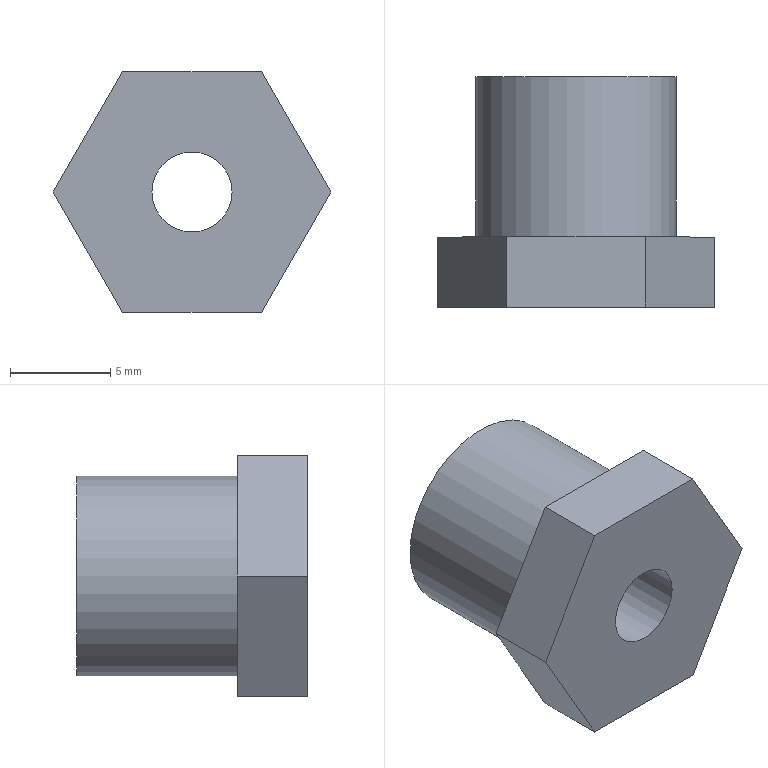Part | STEP file | 1-06.4 | 1 solid | 11 faces | box 13.856 x 11.5 x 12 mm | volume 920.282 mm3 | plane 9 | cylinder 2 | commonest cylinder face diameters 4 x1 10 x1
STEP:
#1=CARTESIAN_POINT('',(0.,0.,0.));
#2=DIRECTION('',(0.,0.,1.));
#3=DIRECTION('',(1.,0.,0.));
#4=AXIS2_PLACEMENT_3D('',#1,#2,#3);
#5=CARTESIAN_POINT('',(-3.464,0.,6.));
#6=VERTEX_POINT('',#5);
#7=CARTESIAN_POINT('',(3.464,0.,6.));
#8=VERTEX_POINT('',#7);
#9=CARTESIAN_POINT('',(-3.464,0.,6.));
#10=DIRECTION('',(1.,0.,0.));
#11=VECTOR('',#10,1.);
#12=LINE('',#9,#11);
#13=CARTESIAN_POINT('',(0.,-1.75,6.));
#14=DIRECTION('',(0.,0.,-1.));
#15=DIRECTION('',(1.,0.,0.));
#16=AXIS2_PLACEMENT_3D('',#13,#14,#15);
#17=PLANE('',#16);
#18=CARTESIAN_POINT('',(-3.464,-1.75));
#19=DIRECTION('',(1.,0.));
#20=VECTOR('',#19,1.);
#21=LINE('',#18,#20);
#22=(GEOMETRIC_REPRESENTATION_CONTEXT(2)PARAMETRIC_REPRESENTATION_CONTEXT()REPRESENTATION_CONTEXT('',''));
#23=DEFINITIONAL_REPRESENTATION('',(#21),#22);
#24=PCURVE('',#17,#23);
#25=CARTESIAN_POINT('',(0.,0.,-0.9282));
#26=DIRECTION('',(0.,1.,0.));
#27=DIRECTION('',(1.,0.,0.));
#28=AXIS2_PLACEMENT_3D('',#25,#26,#27);
#29=PLANE('',#28);
#30=CARTESIAN_POINT('',(-3.464,-6.928));
#31=DIRECTION('',(1.,0.));
#32=VECTOR('',#31,1.);
#33=LINE('',#30,#32);
#34=(GEOMETRIC_REPRESENTATION_CONTEXT(2)PARAMETRIC_REPRESENTATION_CONTEXT()REPRESENTATION_CONTEXT('',''));
#35=DEFINITIONAL_REPRESENTATION('',(#33),#34);
#36=PCURVE('',#29,#35);
#37=SURFACE_CURVE('',#12,(#24,#36),.PCURVE_S1.);
#38=EDGE_CURVE('',#6,#8,#37,.T.);
#39=ORIENTED_EDGE('',*,*,#38,.T.);
#40=CARTESIAN_POINT('',(3.464,-3.5,6.));
#41=VERTEX_POINT('',#40);
#42=CARTESIAN_POINT('',(3.464,0.,6.));
#43=DIRECTION('',(0.,-1.,0.));
#44=VECTOR('',#43,1.);
#45=LINE('',#42,#44);
#46=CARTESIAN_POINT('',(3.464,-1.75));
#47=DIRECTION('',(0.,1.));
#48=VECTOR('',#47,1.);
#49=LINE('',#46,#48);
#50=(GEOMETRIC_REPRESENTATION_CONTEXT(2)PARAMETRIC_REPRESENTATION_CONTEXT()REPRESENTATION_CONTEXT('',''));
#51=DEFINITIONAL_REPRESENTATION('',(#49),#50);
#52=PCURVE('',#17,#51);
#53=CARTESIAN_POINT('',(5.196,-1.75,3.));
#54=DIRECTION('',(-0.866,0.,-0.5));
#55=DIRECTION('',(0.5,0.,-0.866));
#56=AXIS2_PLACEMENT_3D('',#53,#54,#55);
#57=PLANE('',#56);
#58=CARTESIAN_POINT('',(-3.464,-1.75));
#59=DIRECTION('',(0.,1.));
#60=VECTOR('',#59,1.);
#61=LINE('',#58,#60);
#62=(GEOMETRIC_REPRESENTATION_CONTEXT(2)PARAMETRIC_REPRESENTATION_CONTEXT()REPRESENTATION_CONTEXT('',''));
#63=DEFINITIONAL_REPRESENTATION('',(#61),#62);
#64=PCURVE('',#57,#63);
#65=SURFACE_CURVE('',#45,(#52,#64),.PCURVE_S1.);
#66=EDGE_CURVE('',#8,#41,#65,.T.);
#67=ORIENTED_EDGE('',*,*,#66,.T.);
#68=CARTESIAN_POINT('',(-3.464,-3.5,6.));
#69=VERTEX_POINT('',#68);
#70=CARTESIAN_POINT('',(-3.464,-3.5,6.));
#71=DIRECTION('',(1.,0.,0.));
#72=VECTOR('',#71,1.);
#73=LINE('',#70,#72);
#74=CARTESIAN_POINT('',(-3.464,1.75));
#75=DIRECTION('',(1.,0.));
#76=VECTOR('',#75,1.);
#77=LINE('',#74,#76);
#78=(GEOMETRIC_REPRESENTATION_CONTEXT(2)PARAMETRIC_REPRESENTATION_CONTEXT()REPRESENTATION_CONTEXT('',''));
#79=DEFINITIONAL_REPRESENTATION('',(#77),#78);
#80=PCURVE('',#17,#79);
#81=CARTESIAN_POINT('',(0.,-3.5,-0.9282));
#82=DIRECTION('',(0.,1.,0.));
#83=DIRECTION('',(1.,0.,0.));
#84=AXIS2_PLACEMENT_3D('',#81,#82,#83);
#85=PLANE('',#84);
#86=CARTESIAN_POINT('',(-3.464,-6.928));
#87=DIRECTION('',(1.,0.));
#88=VECTOR('',#87,1.);
#89=LINE('',#86,#88);
#90=(GEOMETRIC_REPRESENTATION_CONTEXT(2)PARAMETRIC_REPRESENTATION_CONTEXT()REPRESENTATION_CONTEXT('',''));
#91=DEFINITIONAL_REPRESENTATION('',(#89),#90);
#92=PCURVE('',#85,#91);
#93=SURFACE_CURVE('',#73,(#80,#92),.PCURVE_S1.);
#94=EDGE_CURVE('',#69,#41,#93,.T.);
#95=ORIENTED_EDGE('',*,*,#94,.F.);
#96=CARTESIAN_POINT('',(-3.464,0.,6.));
#97=DIRECTION('',(0.,-1.,0.));
#98=VECTOR('',#97,1.);
#99=LINE('',#96,#98);
#100=CARTESIAN_POINT('',(-3.464,-1.75));
#101=DIRECTION('',(0.,1.));
#102=VECTOR('',#101,1.);
#103=LINE('',#100,#102);
#104=(GEOMETRIC_REPRESENTATION_CONTEXT(2)PARAMETRIC_REPRESENTATION_CONTEXT()REPRESENTATION_CONTEXT('',''));
#105=DEFINITIONAL_REPRESENTATION('',(#103),#104);
#106=PCURVE('',#17,#105);
#107=CARTESIAN_POINT('',(-5.196,-1.75,3.));
#108=DIRECTION('',(0.866,0.,-0.5));
#109=DIRECTION('',(0.5,0.,0.866));
#110=AXIS2_PLACEMENT_3D('',#107,#108,#109);
#111=PLANE('',#110);
#112=CARTESIAN_POINT('',(3.464,-1.75));
#113=DIRECTION('',(0.,1.));
#114=VECTOR('',#113,1.);
#115=LINE('',#112,#114);
#116=(GEOMETRIC_REPRESENTATION_CONTEXT(2)PARAMETRIC_REPRESENTATION_CONTEXT()REPRESENTATION_CONTEXT('',''));
#117=DEFINITIONAL_REPRESENTATION('',(#115),#116);
#118=PCURVE('',#111,#117);
#119=SURFACE_CURVE('',#99,(#106,#118),.PCURVE_S1.);
#120=EDGE_CURVE('',#6,#69,#119,.T.);
#121=ORIENTED_EDGE('',*,*,#120,.F.);
#122=EDGE_LOOP('',(#39,#67,#95,#121));
#123=FACE_BOUND('',#122,.F.);
#124=ADVANCED_FACE('',(#123),#17,.F.);
#125=CARTESIAN_POINT('',(6.928,0.,0.));
#126=VERTEX_POINT('',#125);
#127=CARTESIAN_POINT('',(3.464,0.,6.));
#128=DIRECTION('',(0.5,0.,-0.866));
#129=VECTOR('',#128,1.);
#130=LINE('',#127,#129);
#131=CARTESIAN_POINT('',(-3.464,-1.75));
#132=DIRECTION('',(1.,0.));
#133=VECTOR('',#132,1.);
#134=LINE('',#131,#133);
#135=(GEOMETRIC_REPRESENTATION_CONTEXT(2)PARAMETRIC_REPRESENTATION_CONTEXT()REPRESENTATION_CONTEXT('',''));
#136=DEFINITIONAL_REPRESENTATION('',(#134),#135);
#137=PCURVE('',#57,#136);
#138=CARTESIAN_POINT('',(3.464,-6.928));
#139=DIRECTION('',(0.5,0.866));
#140=VECTOR('',#139,1.);
#141=LINE('',#138,#140);
#142=(GEOMETRIC_REPRESENTATION_CONTEXT(2)PARAMETRIC_REPRESENTATION_CONTEXT()REPRESENTATION_CONTEXT('',''));
#143=DEFINITIONAL_REPRESENTATION('',(#141),#142);
#144=PCURVE('',#29,#143);
#145=SURFACE_CURVE('',#130,(#137,#144),.PCURVE_S1.);
#146=EDGE_CURVE('',#8,#126,#145,.T.);
#147=ORIENTED_EDGE('',*,*,#146,.T.);
#148=CARTESIAN_POINT('',(6.928,-3.5,0.));
#149=VERTEX_POINT('',#148);
#150=CARTESIAN_POINT('',(6.928,0.,0.));
#151=DIRECTION('',(0.,-1.,0.));
#152=VECTOR('',#151,1.);
#153=LINE('',#150,#152);
#154=CARTESIAN_POINT('',(3.464,-1.75));
#155=DIRECTION('',(0.,1.));
#156=VECTOR('',#155,1.);
#157=LINE('',#154,#156);
#158=(GEOMETRIC_REPRESENTATION_CONTEXT(2)PARAMETRIC_REPRESENTATION_CONTEXT()REPRESENTATION_CONTEXT('',''));
#159=DEFINITIONAL_REPRESENTATION('',(#157),#158);
#160=PCURVE('',#57,#159);
#161=CARTESIAN_POINT('',(5.196,-1.75,-3.));
#162=DIRECTION('',(-0.866,0.,0.5));
#163=DIRECTION('',(-0.5,0.,-0.866));
#164=AXIS2_PLACEMENT_3D('',#161,#162,#163);
#165=PLANE('',#164);
#166=CARTESIAN_POINT('',(-3.464,-1.75));
#167=DIRECTION('',(0.,1.));
#168=VECTOR('',#167,1.);
#169=LINE('',#166,#168);
#170=(GEOMETRIC_REPRESENTATION_CONTEXT(2)PARAMETRIC_REPRESENTATION_CONTEXT()REPRESENTATION_CONTEXT('',''));
#171=DEFINITIONAL_REPRESENTATION('',(#169),#170);
#172=PCURVE('',#165,#171);
#173=SURFACE_CURVE('',#153,(#160,#172),.PCURVE_S1.);
#174=EDGE_CURVE('',#126,#149,#173,.T.);
#175=ORIENTED_EDGE('',*,*,#174,.T.);
#176=CARTESIAN_POINT('',(3.464,-3.5,6.));
#177=DIRECTION('',(0.5,0.,-0.866));
#178=VECTOR('',#177,1.);
#179=LINE('',#176,#178);
#180=CARTESIAN_POINT('',(-3.464,1.75));
#181=DIRECTION('',(1.,0.));
#182=VECTOR('',#181,1.);
#183=LINE('',#180,#182);
#184=(GEOMETRIC_REPRESENTATION_CONTEXT(2)PARAMETRIC_REPRESENTATION_CONTEXT()REPRESENTATION_CONTEXT('',''));
#185=DEFINITIONAL_REPRESENTATION('',(#183),#184);
#186=PCURVE('',#57,#185);
#187=CARTESIAN_POINT('',(3.464,-6.928));
#188=DIRECTION('',(0.5,0.866));
#189=VECTOR('',#188,1.);
#190=LINE('',#187,#189);
#191=(GEOMETRIC_REPRESENTATION_CONTEXT(2)PARAMETRIC_REPRESENTATION_CONTEXT()REPRESENTATION_CONTEXT('',''));
#192=DEFINITIONAL_REPRESENTATION('',(#190),#191);
#193=PCURVE('',#85,#192);
#194=SURFACE_CURVE('',#179,(#186,#193),.PCURVE_S1.);
#195=EDGE_CURVE('',#41,#149,#194,.T.);
#196=ORIENTED_EDGE('',*,*,#195,.F.);
#197=ORIENTED_EDGE('',*,*,#66,.F.);
#198=EDGE_LOOP('',(#147,#175,#196,#197));
#199=FACE_BOUND('',#198,.F.);
#200=ADVANCED_FACE('',(#199),#57,.F.);
#201=CARTESIAN_POINT('',(3.464,0.,-6.));
#202=VERTEX_POINT('',#201);
#203=CARTESIAN_POINT('',(6.928,0.,0.));
#204=DIRECTION('',(-0.5,0.,-0.866));
#205=VECTOR('',#204,1.);
#206=LINE('',#203,#205);
#207=CARTESIAN_POINT('',(-3.464,-1.75));
#208=DIRECTION('',(1.,0.));
#209=VECTOR('',#208,1.);
#210=LINE('',#207,#209);
#211=(GEOMETRIC_REPRESENTATION_CONTEXT(2)PARAMETRIC_REPRESENTATION_CONTEXT()REPRESENTATION_CONTEXT('',''));
#212=DEFINITIONAL_REPRESENTATION('',(#210),#211);
#213=PCURVE('',#165,#212);
#214=CARTESIAN_POINT('',(6.928,-0.9282));
#215=DIRECTION('',(-0.5,0.866));
#216=VECTOR('',#215,1.);
#217=LINE('',#214,#216);
#218=(GEOMETRIC_REPRESENTATION_CONTEXT(2)PARAMETRIC_REPRESENTATION_CONTEXT()REPRESENTATION_CONTEXT('',''));
#219=DEFINITIONAL_REPRESENTATION('',(#217),#218);
#220=PCURVE('',#29,#219);
#221=SURFACE_CURVE('',#206,(#213,#220),.PCURVE_S1.);
#222=EDGE_CURVE('',#126,#202,#221,.T.);
#223=ORIENTED_EDGE('',*,*,#222,.T.);
#224=CARTESIAN_POINT('',(3.464,-3.5,-6.));
#225=VERTEX_POINT('',#224);
#226=CARTESIAN_POINT('',(3.464,0.,-6.));
#227=DIRECTION('',(0.,-1.,0.));
#228=VECTOR('',#227,1.);
#229=LINE('',#226,#228);
#230=CARTESIAN_POINT('',(3.464,-1.75));
#231=DIRECTION('',(0.,1.));
#232=VECTOR('',#231,1.);
#233=LINE('',#230,#232);
#234=(GEOMETRIC_REPRESENTATION_CONTEXT(2)PARAMETRIC_REPRESENTATION_CONTEXT()REPRESENTATION_CONTEXT('',''));
#235=DEFINITIONAL_REPRESENTATION('',(#233),#234);
#236=PCURVE('',#165,#235);
#237=CARTESIAN_POINT('',(0.,-1.75,-6.));
#238=DIRECTION('',(0.,0.,1.));
#239=DIRECTION('',(-1.,0.,0.));
#240=AXIS2_PLACEMENT_3D('',#237,#238,#239);
#241=PLANE('',#240);
#242=CARTESIAN_POINT('',(-3.464,-1.75));
#243=DIRECTION('',(0.,1.));
#244=VECTOR('',#243,1.);
#245=LINE('',#242,#244);
#246=(GEOMETRIC_REPRESENTATION_CONTEXT(2)PARAMETRIC_REPRESENTATION_CONTEXT()REPRESENTATION_CONTEXT('',''));
#247=DEFINITIONAL_REPRESENTATION('',(#245),#246);
#248=PCURVE('',#241,#247);
#249=SURFACE_CURVE('',#229,(#236,#248),.PCURVE_S1.);
#250=EDGE_CURVE('',#202,#225,#249,.T.);
#251=ORIENTED_EDGE('',*,*,#250,.T.);
#252=CARTESIAN_POINT('',(6.928,-3.5,0.));
#253=DIRECTION('',(-0.5,0.,-0.866));
#254=VECTOR('',#253,1.);
#255=LINE('',#252,#254);
#256=CARTESIAN_POINT('',(-3.464,1.75));
#257=DIRECTION('',(1.,0.));
#258=VECTOR('',#257,1.);
#259=LINE('',#256,#258);
#260=(GEOMETRIC_REPRESENTATION_CONTEXT(2)PARAMETRIC_REPRESENTATION_CONTEXT()REPRESENTATION_CONTEXT('',''));
#261=DEFINITIONAL_REPRESENTATION('',(#259),#260);
#262=PCURVE('',#165,#261);
#263=CARTESIAN_POINT('',(6.928,-0.9282));
#264=DIRECTION('',(-0.5,0.866));
#265=VECTOR('',#264,1.);
#266=LINE('',#263,#265);
#267=(GEOMETRIC_REPRESENTATION_CONTEXT(2)PARAMETRIC_REPRESENTATION_CONTEXT()REPRESENTATION_CONTEXT('',''));
#268=DEFINITIONAL_REPRESENTATION('',(#266),#267);
#269=PCURVE('',#85,#268);
#270=SURFACE_CURVE('',#255,(#262,#269),.PCURVE_S1.);
#271=EDGE_CURVE('',#149,#225,#270,.T.);
#272=ORIENTED_EDGE('',*,*,#271,.F.);
#273=ORIENTED_EDGE('',*,*,#174,.F.);
#274=EDGE_LOOP('',(#223,#251,#272,#273));
#275=FACE_BOUND('',#274,.F.);
#276=ADVANCED_FACE('',(#275),#165,.F.);
#277=CARTESIAN_POINT('',(-3.464,0.,-6.));
#278=VERTEX_POINT('',#277);
#279=CARTESIAN_POINT('',(3.464,0.,-6.));
#280=DIRECTION('',(-1.,0.,0.));
#281=VECTOR('',#280,1.);
#282=LINE('',#279,#281);
#283=CARTESIAN_POINT('',(-3.464,-1.75));
#284=DIRECTION('',(1.,0.));
#285=VECTOR('',#284,1.);
#286=LINE('',#283,#285);
#287=(GEOMETRIC_REPRESENTATION_CONTEXT(2)PARAMETRIC_REPRESENTATION_CONTEXT()REPRESENTATION_CONTEXT('',''));
#288=DEFINITIONAL_REPRESENTATION('',(#286),#287);
#289=PCURVE('',#241,#288);
#290=CARTESIAN_POINT('',(3.464,5.072));
#291=DIRECTION('',(-1.,0.));
#292=VECTOR('',#291,1.);
#293=LINE('',#290,#292);
#294=(GEOMETRIC_REPRESENTATION_CONTEXT(2)PARAMETRIC_REPRESENTATION_CONTEXT()REPRESENTATION_CONTEXT('',''));
#295=DEFINITIONAL_REPRESENTATION('',(#293),#294);
#296=PCURVE('',#29,#295);
#297=SURFACE_CURVE('',#282,(#289,#296),.PCURVE_S1.);
#298=EDGE_CURVE('',#202,#278,#297,.T.);
#299=ORIENTED_EDGE('',*,*,#298,.T.);
#300=CARTESIAN_POINT('',(-3.464,-3.5,-6.));
#301=VERTEX_POINT('',#300);
#302=CARTESIAN_POINT('',(-3.464,0.,-6.));
#303=DIRECTION('',(0.,-1.,0.));
#304=VECTOR('',#303,1.);
#305=LINE('',#302,#304);
#306=CARTESIAN_POINT('',(3.464,-1.75));
#307=DIRECTION('',(0.,1.));
#308=VECTOR('',#307,1.);
#309=LINE('',#306,#308);
#310=(GEOMETRIC_REPRESENTATION_CONTEXT(2)PARAMETRIC_REPRESENTATION_CONTEXT()REPRESENTATION_CONTEXT('',''));
#311=DEFINITIONAL_REPRESENTATION('',(#309),#310);
#312=PCURVE('',#241,#311);
#313=CARTESIAN_POINT('',(-5.196,-1.75,-3.));
#314=DIRECTION('',(0.866,0.,0.5));
#315=DIRECTION('',(-0.5,0.,0.866));
#316=AXIS2_PLACEMENT_3D('',#313,#314,#315);
#317=PLANE('',#316);
#318=CARTESIAN_POINT('',(-3.464,-1.75));
#319=DIRECTION('',(0.,1.));
#320=VECTOR('',#319,1.);
#321=LINE('',#318,#320);
#322=(GEOMETRIC_REPRESENTATION_CONTEXT(2)PARAMETRIC_REPRESENTATION_CONTEXT()REPRESENTATION_CONTEXT('',''));
#323=DEFINITIONAL_REPRESENTATION('',(#321),#322);
#324=PCURVE('',#317,#323);
#325=SURFACE_CURVE('',#305,(#312,#324),.PCURVE_S1.);
#326=EDGE_CURVE('',#278,#301,#325,.T.);
#327=ORIENTED_EDGE('',*,*,#326,.T.);
#328=CARTESIAN_POINT('',(3.464,-3.5,-6.));
#329=DIRECTION('',(-1.,0.,0.));
#330=VECTOR('',#329,1.);
#331=LINE('',#328,#330);
#332=CARTESIAN_POINT('',(-3.464,1.75));
#333=DIRECTION('',(1.,0.));
#334=VECTOR('',#333,1.);
#335=LINE('',#332,#334);
#336=(GEOMETRIC_REPRESENTATION_CONTEXT(2)PARAMETRIC_REPRESENTATION_CONTEXT()REPRESENTATION_CONTEXT('',''));
#337=DEFINITIONAL_REPRESENTATION('',(#335),#336);
#338=PCURVE('',#241,#337);
#339=CARTESIAN_POINT('',(3.464,5.072));
#340=DIRECTION('',(-1.,0.));
#341=VECTOR('',#340,1.);
#342=LINE('',#339,#341);
#343=(GEOMETRIC_REPRESENTATION_CONTEXT(2)PARAMETRIC_REPRESENTATION_CONTEXT()REPRESENTATION_CONTEXT('',''));
#344=DEFINITIONAL_REPRESENTATION('',(#342),#343);
#345=PCURVE('',#85,#344);
#346=SURFACE_CURVE('',#331,(#338,#345),.PCURVE_S1.);
#347=EDGE_CURVE('',#225,#301,#346,.T.);
#348=ORIENTED_EDGE('',*,*,#347,.F.);
#349=ORIENTED_EDGE('',*,*,#250,.F.);
#350=EDGE_LOOP('',(#299,#327,#348,#349));
#351=FACE_BOUND('',#350,.F.);
#352=ADVANCED_FACE('',(#351),#241,.F.);
#353=CARTESIAN_POINT('',(-6.928,0.,0.));
#354=VERTEX_POINT('',#353);
#355=CARTESIAN_POINT('',(-3.464,0.,-6.));
#356=DIRECTION('',(-0.5,0.,0.866));
#357=VECTOR('',#356,1.);
#358=LINE('',#355,#357);
#359=CARTESIAN_POINT('',(-3.464,-1.75));
#360=DIRECTION('',(1.,0.));
#361=VECTOR('',#360,1.);
#362=LINE('',#359,#361);
#363=(GEOMETRIC_REPRESENTATION_CONTEXT(2)PARAMETRIC_REPRESENTATION_CONTEXT()REPRESENTATION_CONTEXT('',''));
#364=DEFINITIONAL_REPRESENTATION('',(#362),#363);
#365=PCURVE('',#317,#364);
#366=CARTESIAN_POINT('',(-3.464,5.072));
#367=DIRECTION('',(-0.5,-0.866));
#368=VECTOR('',#367,1.);
#369=LINE('',#366,#368);
#370=(GEOMETRIC_REPRESENTATION_CONTEXT(2)PARAMETRIC_REPRESENTATION_CONTEXT()REPRESENTATION_CONTEXT('',''));
#371=DEFINITIONAL_REPRESENTATION('',(#369),#370);
#372=PCURVE('',#29,#371);
#373=SURFACE_CURVE('',#358,(#365,#372),.PCURVE_S1.);
#374=EDGE_CURVE('',#278,#354,#373,.T.);
#375=ORIENTED_EDGE('',*,*,#374,.T.);
#376=CARTESIAN_POINT('',(-6.928,-3.5,0.));
#377=VERTEX_POINT('',#376);
#378=CARTESIAN_POINT('',(-6.928,0.,0.));
#379=DIRECTION('',(0.,-1.,0.));
#380=VECTOR('',#379,1.);
#381=LINE('',#378,#380);
#382=CARTESIAN_POINT('',(3.464,-1.75));
#383=DIRECTION('',(0.,1.));
#384=VECTOR('',#383,1.);
#385=LINE('',#382,#384);
#386=(GEOMETRIC_REPRESENTATION_CONTEXT(2)PARAMETRIC_REPRESENTATION_CONTEXT()REPRESENTATION_CONTEXT('',''));
#387=DEFINITIONAL_REPRESENTATION('',(#385),#386);
#388=PCURVE('',#317,#387);
#389=CARTESIAN_POINT('',(-3.464,-1.75));
#390=DIRECTION('',(0.,1.));
#391=VECTOR('',#390,1.);
#392=LINE('',#389,#391);
#393=(GEOMETRIC_REPRESENTATION_CONTEXT(2)PARAMETRIC_REPRESENTATION_CONTEXT()REPRESENTATION_CONTEXT('',''));
#394=DEFINITIONAL_REPRESENTATION('',(#392),#393);
#395=PCURVE('',#111,#394);
#396=SURFACE_CURVE('',#381,(#388,#395),.PCURVE_S1.);
#397=EDGE_CURVE('',#354,#377,#396,.T.);
#398=ORIENTED_EDGE('',*,*,#397,.T.);
#399=CARTESIAN_POINT('',(-3.464,-3.5,-6.));
#400=DIRECTION('',(-0.5,0.,0.866));
#401=VECTOR('',#400,1.);
#402=LINE('',#399,#401);
#403=CARTESIAN_POINT('',(-3.464,1.75));
#404=DIRECTION('',(1.,0.));
#405=VECTOR('',#404,1.);
#406=LINE('',#403,#405);
#407=(GEOMETRIC_REPRESENTATION_CONTEXT(2)PARAMETRIC_REPRESENTATION_CONTEXT()REPRESENTATION_CONTEXT('',''));
#408=DEFINITIONAL_REPRESENTATION('',(#406),#407);
#409=PCURVE('',#317,#408);
#410=CARTESIAN_POINT('',(-3.464,5.072));
#411=DIRECTION('',(-0.5,-0.866));
#412=VECTOR('',#411,1.);
#413=LINE('',#410,#412);
#414=(GEOMETRIC_REPRESENTATION_CONTEXT(2)PARAMETRIC_REPRESENTATION_CONTEXT()REPRESENTATION_CONTEXT('',''));
#415=DEFINITIONAL_REPRESENTATION('',(#413),#414);
#416=PCURVE('',#85,#415);
#417=SURFACE_CURVE('',#402,(#409,#416),.PCURVE_S1.);
#418=EDGE_CURVE('',#301,#377,#417,.T.);
#419=ORIENTED_EDGE('',*,*,#418,.F.);
#420=ORIENTED_EDGE('',*,*,#326,.F.);
#421=EDGE_LOOP('',(#375,#398,#419,#420));
#422=FACE_BOUND('',#421,.F.);
#423=ADVANCED_FACE('',(#422),#317,.F.);
#424=CARTESIAN_POINT('',(-6.928,0.,0.));
#425=DIRECTION('',(0.5,0.,0.866));
#426=VECTOR('',#425,1.);
#427=LINE('',#424,#426);
#428=CARTESIAN_POINT('',(-3.464,-1.75));
#429=DIRECTION('',(1.,0.));
#430=VECTOR('',#429,1.);
#431=LINE('',#428,#430);
#432=(GEOMETRIC_REPRESENTATION_CONTEXT(2)PARAMETRIC_REPRESENTATION_CONTEXT()REPRESENTATION_CONTEXT('',''));
#433=DEFINITIONAL_REPRESENTATION('',(#431),#432);
#434=PCURVE('',#111,#433);
#435=CARTESIAN_POINT('',(-6.928,-0.9282));
#436=DIRECTION('',(0.5,-0.866));
#437=VECTOR('',#436,1.);
#438=LINE('',#435,#437);
#439=(GEOMETRIC_REPRESENTATION_CONTEXT(2)PARAMETRIC_REPRESENTATION_CONTEXT()REPRESENTATION_CONTEXT('',''));
#440=DEFINITIONAL_REPRESENTATION('',(#438),#439);
#441=PCURVE('',#29,#440);
#442=SURFACE_CURVE('',#427,(#434,#441),.PCURVE_S1.);
#443=EDGE_CURVE('',#354,#6,#442,.T.);
#444=ORIENTED_EDGE('',*,*,#443,.T.);
#445=ORIENTED_EDGE('',*,*,#120,.T.);
#446=CARTESIAN_POINT('',(-6.928,-3.5,0.));
#447=DIRECTION('',(0.5,0.,0.866));
#448=VECTOR('',#447,1.);
#449=LINE('',#446,#448);
#450=CARTESIAN_POINT('',(-3.464,1.75));
#451=DIRECTION('',(1.,0.));
#452=VECTOR('',#451,1.);
#453=LINE('',#450,#452);
#454=(GEOMETRIC_REPRESENTATION_CONTEXT(2)PARAMETRIC_REPRESENTATION_CONTEXT()REPRESENTATION_CONTEXT('',''));
#455=DEFINITIONAL_REPRESENTATION('',(#453),#454);
#456=PCURVE('',#111,#455);
#457=CARTESIAN_POINT('',(-6.928,-0.9282));
#458=DIRECTION('',(0.5,-0.866));
#459=VECTOR('',#458,1.);
#460=LINE('',#457,#459);
#461=(GEOMETRIC_REPRESENTATION_CONTEXT(2)PARAMETRIC_REPRESENTATION_CONTEXT()REPRESENTATION_CONTEXT('',''));
#462=DEFINITIONAL_REPRESENTATION('',(#460),#461);
#463=PCURVE('',#85,#462);
#464=SURFACE_CURVE('',#449,(#456,#463),.PCURVE_S1.);
#465=EDGE_CURVE('',#377,#69,#464,.T.);
#466=ORIENTED_EDGE('',*,*,#465,.F.);
#467=ORIENTED_EDGE('',*,*,#397,.F.);
#468=EDGE_LOOP('',(#444,#445,#466,#467));
#469=FACE_BOUND('',#468,.F.);
#470=ADVANCED_FACE('',(#469),#111,.F.);
#471=ORIENTED_EDGE('',*,*,#38,.T.);
#472=ORIENTED_EDGE('',*,*,#146,.T.);
#473=ORIENTED_EDGE('',*,*,#222,.T.);
#474=ORIENTED_EDGE('',*,*,#298,.T.);
#475=ORIENTED_EDGE('',*,*,#374,.T.);
#476=ORIENTED_EDGE('',*,*,#443,.T.);
#477=EDGE_LOOP('',(#471,#472,#473,#474,#475,#476));
#478=FACE_BOUND('',#477,.T.);
#479=CARTESIAN_POINT('',(5.,0.,0.));
#480=VERTEX_POINT('',#479);
#481=CARTESIAN_POINT('',(0.,0.,0.));
#482=DIRECTION('',(0.,-1.,0.));
#483=DIRECTION('',(1.,0.,0.));
#484=AXIS2_PLACEMENT_3D('',#481,#482,#483);
#485=CIRCLE('',#484,5.);
#486=CARTESIAN_POINT('',(5.,-0.9282));
#487=CARTESIAN_POINT('',(5.,-9.588));
#488=CARTESIAN_POINT('',(-2.5,-5.258));
#489=CARTESIAN_POINT('',(-10.,-0.9282));
#490=CARTESIAN_POINT('',(-2.5,3.402));
#491=CARTESIAN_POINT('',(5.,7.732));
#492=CARTESIAN_POINT('',(5.,-0.9282));
#493=(BOUNDED_CURVE()B_SPLINE_CURVE(2,(#486,#487,#488,#489,#490,#491,#492),.UNSPECIFIED.,.T.,.F.)B_SPLINE_CURVE_WITH_KNOTS((1,2,2,2,2,1),(-2.094,0.,2.094,4.189,6.283,8.378),.UNSPECIFIED.)CURVE()GEOMETRIC_REPRESENTATION_ITEM()RATIONAL_B_SPLINE_CURVE((1.,0.5,1.,0.5,1.,0.5,1.))REPRESENTATION_ITEM(''));
#494=(GEOMETRIC_REPRESENTATION_CONTEXT(2)PARAMETRIC_REPRESENTATION_CONTEXT()REPRESENTATION_CONTEXT('',''));
#495=DEFINITIONAL_REPRESENTATION('',(#493),#494);
#496=PCURVE('',#29,#495);
#497=CARTESIAN_POINT('',(0.,0.,0.));
#498=DIRECTION('',(0.,1.,0.));
#499=DIRECTION('',(1.,0.,0.));
#500=AXIS2_PLACEMENT_3D('',#497,#498,#499);
#501=CYLINDRICAL_SURFACE('',#500,5.);
#502=CARTESIAN_POINT('',(6.283,0.));
#503=DIRECTION('',(-1.,0.));
#504=VECTOR('',#503,1.);
#505=LINE('',#502,#504);
#506=(GEOMETRIC_REPRESENTATION_CONTEXT(2)PARAMETRIC_REPRESENTATION_CONTEXT()REPRESENTATION_CONTEXT('',''));
#507=DEFINITIONAL_REPRESENTATION('',(#505),#506);
#508=PCURVE('',#501,#507);
#509=SURFACE_CURVE('',#485,(#496,#508),.PCURVE_S1.);
#510=EDGE_CURVE('',#480,#480,#509,.T.);
#511=ORIENTED_EDGE('',*,*,#510,.T.);
#512=EDGE_LOOP('',(#511));
#513=FACE_BOUND('',#512,.T.);
#514=ADVANCED_FACE('',(#478,#513),#29,.T.);
#515=CARTESIAN_POINT('',(5.,8.,0.));
#516=VERTEX_POINT('',#515);
#517=CARTESIAN_POINT('',(5.,0.,0.));
#518=DIRECTION('',(0.,1.,0.));
#519=VECTOR('',#518,1.);
#520=LINE('',#517,#519);
#521=CARTESIAN_POINT('',(6.283,0.));
#522=DIRECTION('',(0.,1.));
#523=VECTOR('',#522,1.);
#524=LINE('',#521,#523);
#525=(GEOMETRIC_REPRESENTATION_CONTEXT(2)PARAMETRIC_REPRESENTATION_CONTEXT()REPRESENTATION_CONTEXT('',''));
#526=DEFINITIONAL_REPRESENTATION('',(#524),#525);
#527=PCURVE('',#501,#526);
#528=CARTESIAN_POINT('',(0.,0.));
#529=DIRECTION('',(0.,1.));
#530=VECTOR('',#529,1.);
#531=LINE('',#528,#530);
#532=(GEOMETRIC_REPRESENTATION_CONTEXT(2)PARAMETRIC_REPRESENTATION_CONTEXT()REPRESENTATION_CONTEXT('',''));
#533=DEFINITIONAL_REPRESENTATION('',(#531),#532);
#534=PCURVE('',#501,#533);
#535=SEAM_CURVE('',#520,(#527,#534),.PCURVE_S1.);
#536=EDGE_CURVE('',#480,#516,#535,.T.);
#537=ORIENTED_EDGE('',*,*,#536,.T.);
#538=CARTESIAN_POINT('',(0.,8.,0.));
#539=DIRECTION('',(0.,-1.,0.));
#540=DIRECTION('',(1.,0.,0.));
#541=AXIS2_PLACEMENT_3D('',#538,#539,#540);
#542=CIRCLE('',#541,5.);
#543=CARTESIAN_POINT('',(6.283,8.));
#544=DIRECTION('',(-1.,0.));
#545=VECTOR('',#544,1.);
#546=LINE('',#543,#545);
#547=(GEOMETRIC_REPRESENTATION_CONTEXT(2)PARAMETRIC_REPRESENTATION_CONTEXT()REPRESENTATION_CONTEXT('',''));
#548=DEFINITIONAL_REPRESENTATION('',(#546),#547);
#549=PCURVE('',#501,#548);
#550=CARTESIAN_POINT('',(-1.34,8.,0.));
#551=DIRECTION('',(0.,-1.,0.));
#552=DIRECTION('',(1.,0.,0.));
#553=AXIS2_PLACEMENT_3D('',#550,#551,#552);
#554=PLANE('',#553);
#555=CARTESIAN_POINT('',(1.34,0.));
#556=DIRECTION('',(1.,0.));
#557=AXIS2_PLACEMENT_2D('',#555,#556);
#558=CIRCLE('',#557,5.);
#559=(GEOMETRIC_REPRESENTATION_CONTEXT(2)PARAMETRIC_REPRESENTATION_CONTEXT()REPRESENTATION_CONTEXT('',''));
#560=DEFINITIONAL_REPRESENTATION('',(#558),#559);
#561=PCURVE('',#554,#560);
#562=SURFACE_CURVE('',#542,(#549,#561),.PCURVE_S1.);
#563=EDGE_CURVE('',#516,#516,#562,.T.);
#564=ORIENTED_EDGE('',*,*,#563,.T.);
#565=ORIENTED_EDGE('',*,*,#536,.F.);
#566=ORIENTED_EDGE('',*,*,#510,.F.);
#567=EDGE_LOOP('',(#537,#564,#565,#566));
#568=FACE_BOUND('',#567,.T.);
#569=ADVANCED_FACE('',(#568),#501,.T.);
#570=ORIENTED_EDGE('',*,*,#94,.T.);
#571=ORIENTED_EDGE('',*,*,#195,.T.);
#572=ORIENTED_EDGE('',*,*,#271,.T.);
#573=ORIENTED_EDGE('',*,*,#347,.T.);
#574=ORIENTED_EDGE('',*,*,#418,.T.);
#575=ORIENTED_EDGE('',*,*,#465,.T.);
#576=EDGE_LOOP('',(#570,#571,#572,#573,#574,#575));
#577=FACE_BOUND('',#576,.F.);
#578=CARTESIAN_POINT('',(2.,-3.5,0.));
#579=VERTEX_POINT('',#578);
#580=CARTESIAN_POINT('',(0.,-3.5,0.));
#581=DIRECTION('',(0.,-1.,0.));
#582=DIRECTION('',(1.,0.,0.));
#583=AXIS2_PLACEMENT_3D('',#580,#581,#582);
#584=CIRCLE('',#583,2.);
#585=CARTESIAN_POINT('',(2.,-0.9282));
#586=CARTESIAN_POINT('',(2.,-4.392));
#587=CARTESIAN_POINT('',(-1.,-2.66));
#588=CARTESIAN_POINT('',(-4.,-0.9282));
#589=CARTESIAN_POINT('',(-1.,0.8038));
#590=CARTESIAN_POINT('',(2.,2.536));
#591=CARTESIAN_POINT('',(2.,-0.9282));
#592=(BOUNDED_CURVE()B_SPLINE_CURVE(2,(#585,#586,#587,#588,#589,#590,#591),.UNSPECIFIED.,.T.,.F.)B_SPLINE_CURVE_WITH_KNOTS((1,2,2,2,2,1),(-2.094,0.,2.094,4.189,6.283,8.378),.UNSPECIFIED.)CURVE()GEOMETRIC_REPRESENTATION_ITEM()RATIONAL_B_SPLINE_CURVE((1.,0.5,1.,0.5,1.,0.5,1.))REPRESENTATION_ITEM(''));
#593=(GEOMETRIC_REPRESENTATION_CONTEXT(2)PARAMETRIC_REPRESENTATION_CONTEXT()REPRESENTATION_CONTEXT('',''));
#594=DEFINITIONAL_REPRESENTATION('',(#592),#593);
#595=PCURVE('',#85,#594);
#596=CARTESIAN_POINT('',(0.,-3.5,0.));
#597=DIRECTION('',(0.,1.,0.));
#598=DIRECTION('',(1.,0.,0.));
#599=AXIS2_PLACEMENT_3D('',#596,#597,#598);
#600=CYLINDRICAL_SURFACE('',#599,2.);
#601=CARTESIAN_POINT('',(6.283,0.));
#602=DIRECTION('',(-1.,0.));
#603=VECTOR('',#602,1.);
#604=LINE('',#601,#603);
#605=(GEOMETRIC_REPRESENTATION_CONTEXT(2)PARAMETRIC_REPRESENTATION_CONTEXT()REPRESENTATION_CONTEXT('',''));
#606=DEFINITIONAL_REPRESENTATION('',(#604),#605);
#607=PCURVE('',#600,#606);
#608=SURFACE_CURVE('',#584,(#595,#607),.PCURVE_S1.);
#609=EDGE_CURVE('',#579,#579,#608,.T.);
#610=ORIENTED_EDGE('',*,*,#609,.T.);
#611=EDGE_LOOP('',(#610));
#612=FACE_BOUND('',#611,.F.);
#613=ADVANCED_FACE('',(#577,#612),#85,.F.);
#614=ORIENTED_EDGE('',*,*,#563,.T.);
#615=EDGE_LOOP('',(#614));
#616=FACE_BOUND('',#615,.F.);
#617=CARTESIAN_POINT('',(2.,8.,0.));
#618=VERTEX_POINT('',#617);
#619=CARTESIAN_POINT('',(0.,8.,0.));
#620=DIRECTION('',(0.,1.,0.));
#621=DIRECTION('',(1.,0.,0.));
#622=AXIS2_PLACEMENT_3D('',#619,#620,#621);
#623=CIRCLE('',#622,2.);
#624=CARTESIAN_POINT('',(3.34,0.));
#625=CARTESIAN_POINT('',(3.34,-3.464));
#626=CARTESIAN_POINT('',(0.3397,-1.732));
#627=CARTESIAN_POINT('',(-2.66,0.));
#628=CARTESIAN_POINT('',(0.3397,1.732));
#629=CARTESIAN_POINT('',(3.34,3.464));
#630=CARTESIAN_POINT('',(3.34,0.));
#631=(BOUNDED_CURVE()B_SPLINE_CURVE(2,(#624,#625,#626,#627,#628,#629,#630),.UNSPECIFIED.,.T.,.F.)B_SPLINE_CURVE_WITH_KNOTS((1,2,2,2,2,1),(-2.094,0.,2.094,4.189,6.283,8.378),.UNSPECIFIED.)CURVE()GEOMETRIC_REPRESENTATION_ITEM()RATIONAL_B_SPLINE_CURVE((1.,0.5,1.,0.5,1.,0.5,1.))REPRESENTATION_ITEM(''));
#632=(GEOMETRIC_REPRESENTATION_CONTEXT(2)PARAMETRIC_REPRESENTATION_CONTEXT()REPRESENTATION_CONTEXT('',''));
#633=DEFINITIONAL_REPRESENTATION('',(#631),#632);
#634=PCURVE('',#554,#633);
#635=CARTESIAN_POINT('',(0.,11.5));
#636=DIRECTION('',(1.,0.));
#637=VECTOR('',#636,1.);
#638=LINE('',#635,#637);
#639=(GEOMETRIC_REPRESENTATION_CONTEXT(2)PARAMETRIC_REPRESENTATION_CONTEXT()REPRESENTATION_CONTEXT('',''));
#640=DEFINITIONAL_REPRESENTATION('',(#638),#639);
#641=PCURVE('',#600,#640);
#642=SURFACE_CURVE('',#623,(#634,#641),.PCURVE_S1.);
#643=EDGE_CURVE('',#618,#618,#642,.T.);
#644=ORIENTED_EDGE('',*,*,#643,.T.);
#645=EDGE_LOOP('',(#644));
#646=FACE_BOUND('',#645,.F.);
#647=ADVANCED_FACE('',(#616,#646),#554,.F.);
#648=CARTESIAN_POINT('',(2.,-3.5,0.));
#649=DIRECTION('',(0.,1.,0.));
#650=VECTOR('',#649,1.);
#651=LINE('',#648,#650);
#652=CARTESIAN_POINT('',(6.283,0.));
#653=DIRECTION('',(0.,1.));
#654=VECTOR('',#653,1.);
#655=LINE('',#652,#654);
#656=(GEOMETRIC_REPRESENTATION_CONTEXT(2)PARAMETRIC_REPRESENTATION_CONTEXT()REPRESENTATION_CONTEXT('',''));
#657=DEFINITIONAL_REPRESENTATION('',(#655),#656);
#658=PCURVE('',#600,#657);
#659=CARTESIAN_POINT('',(0.,0.));
#660=DIRECTION('',(0.,1.));
#661=VECTOR('',#660,1.);
#662=LINE('',#659,#661);
#663=(GEOMETRIC_REPRESENTATION_CONTEXT(2)PARAMETRIC_REPRESENTATION_CONTEXT()REPRESENTATION_CONTEXT('',''));
#664=DEFINITIONAL_REPRESENTATION('',(#662),#663);
#665=PCURVE('',#600,#664);
#666=SEAM_CURVE('',#651,(#658,#665),.PCURVE_S1.);
#667=EDGE_CURVE('',#579,#618,#666,.T.);
#668=ORIENTED_EDGE('',*,*,#667,.T.);
#669=ORIENTED_EDGE('',*,*,#643,.F.);
#670=ORIENTED_EDGE('',*,*,#667,.F.);
#671=ORIENTED_EDGE('',*,*,#609,.F.);
#672=EDGE_LOOP('',(#668,#669,#670,#671));
#673=FACE_BOUND('',#672,.F.);
#674=ADVANCED_FACE('',(#673),#600,.F.);
#675=CLOSED_SHELL('',(#124,#200,#276,#352,#423,#470,#514,#569,#613,#647,#674));
#676=MANIFOLD_SOLID_BREP('',#675);
#677=(LENGTH_UNIT()NAMED_UNIT(*)SI_UNIT(.MILLI.,.METRE.));
#678=UNCERTAINTY_MEASURE_WITH_UNIT(LENGTH_MEASURE(0.0000001),#677,'','');
#679=(NAMED_UNIT(*)PLANE_ANGLE_UNIT()SI_UNIT($,.RADIAN.));
#680=(NAMED_UNIT(*)SI_UNIT($,.STERADIAN.)SOLID_ANGLE_UNIT());
#681=(GEOMETRIC_REPRESENTATION_CONTEXT(3)GLOBAL_UNCERTAINTY_ASSIGNED_CONTEXT((#678))GLOBAL_UNIT_ASSIGNED_CONTEXT((#677,#679,#680))REPRESENTATION_CONTEXT('',''));
#682=ADVANCED_BREP_SHAPE_REPRESENTATION('',(#4,#676),#681);